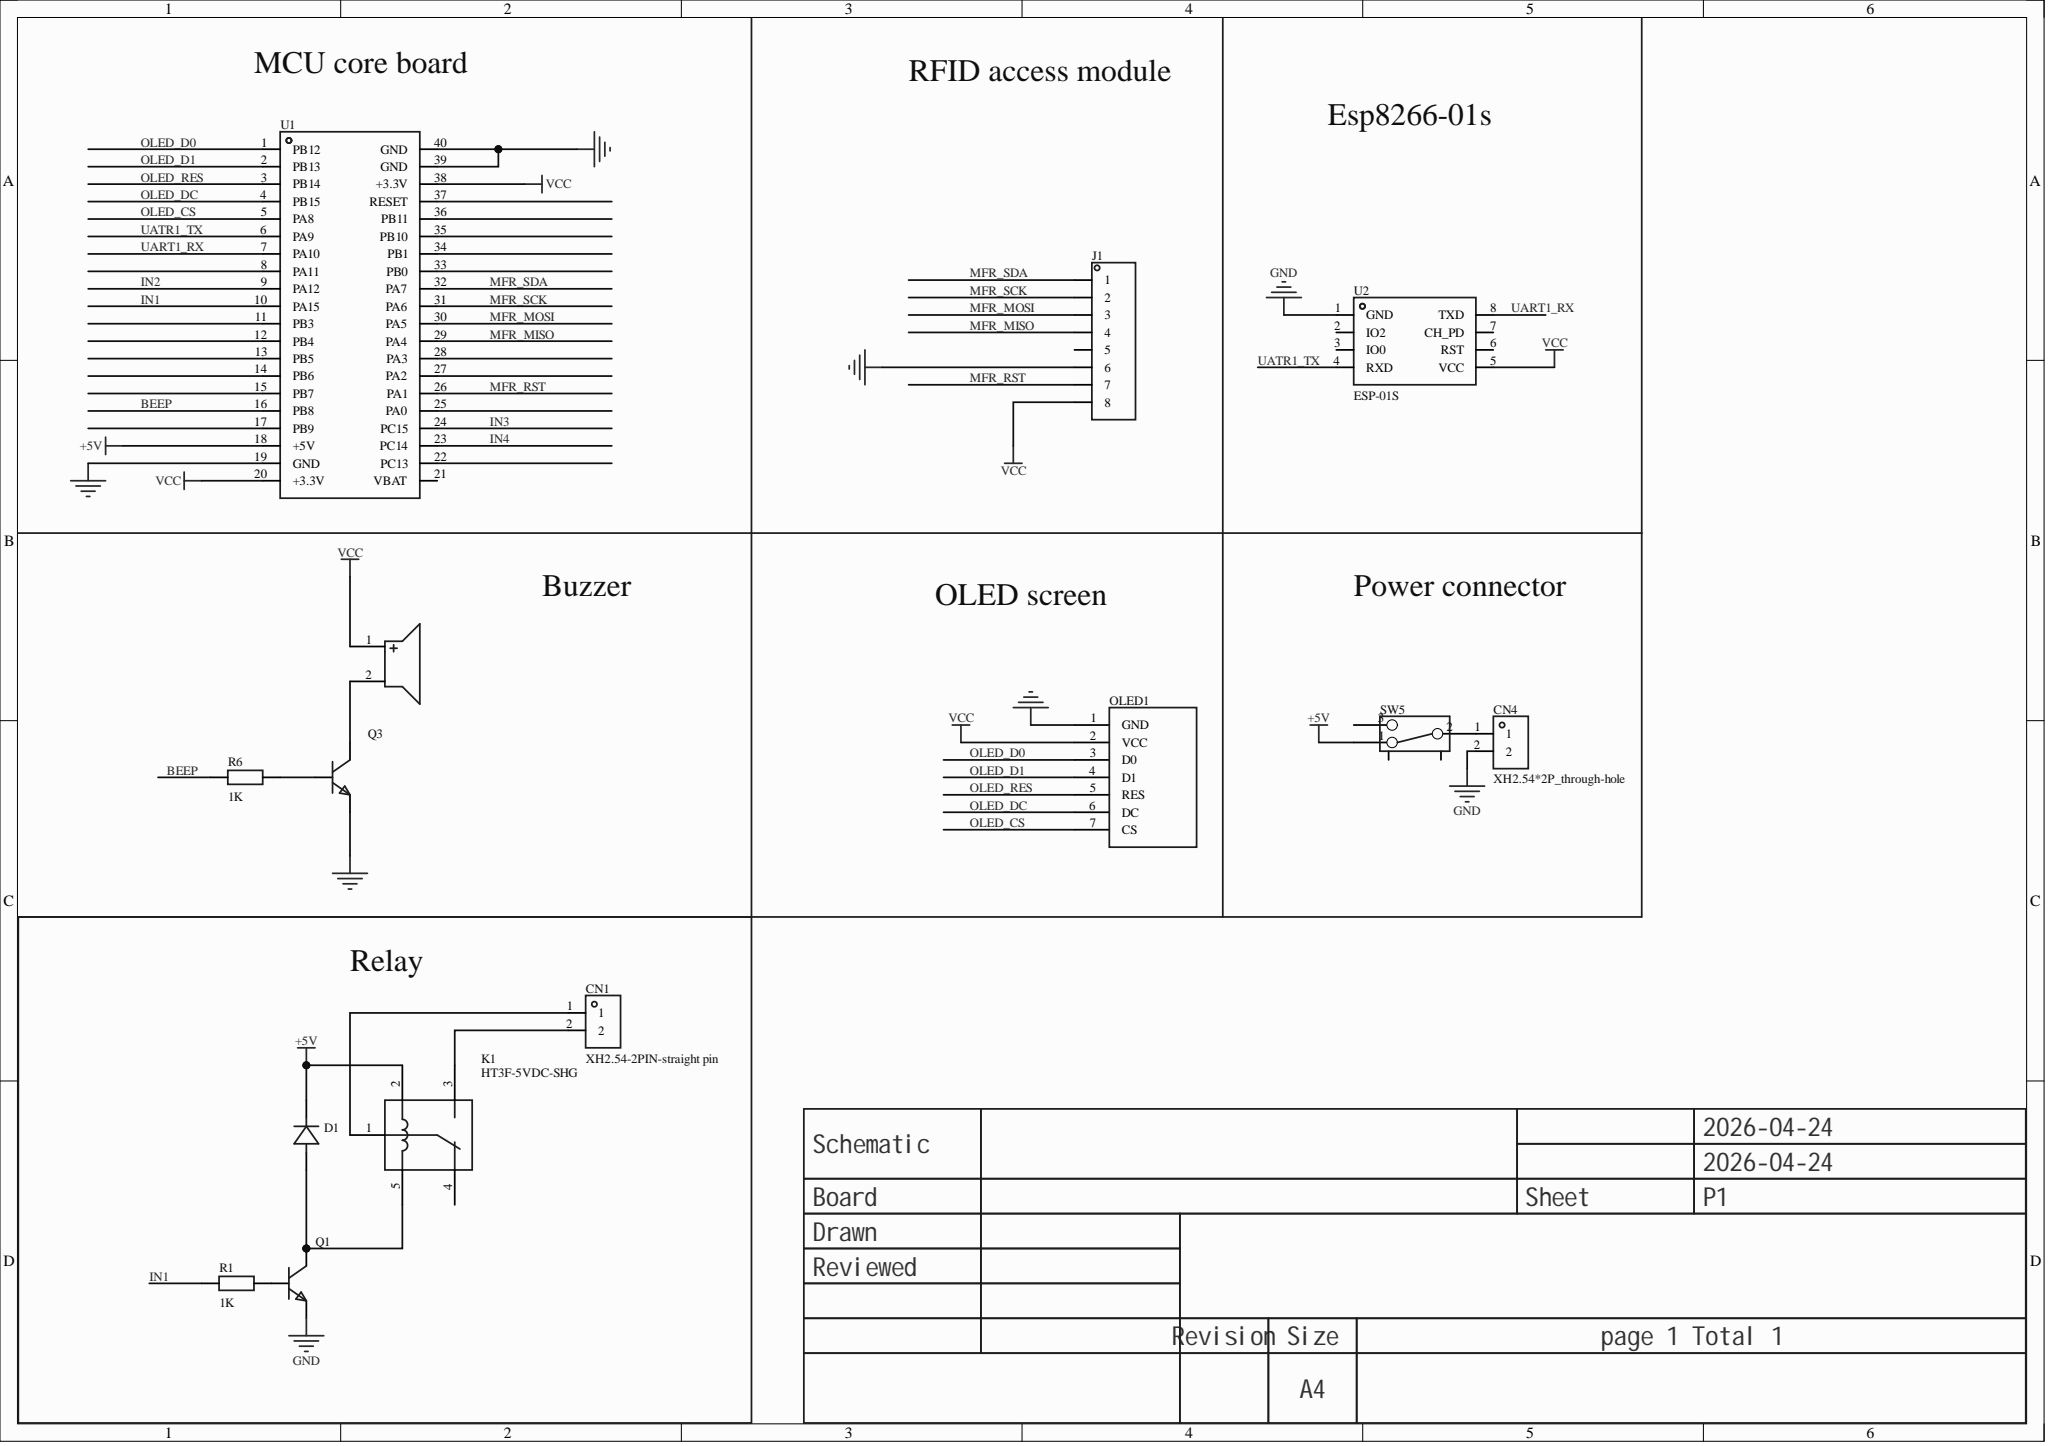Circuit board | Altium Designer | 14 parts | 24 nets
Bill of materials:
Comment,Description,Designator,Footprint,LibRef,Quantity
"2.7kHz","Drive: passive (external drive); type: electromagnetic; frequency: 2.7kHz; SPL: 85dB;","BUZZER1","BUZ-TH_BD9.0-P4.00-D0.6-FD","QMB-09B-03","1"
"XH2.54-2PIN-straight pin","","CN1","CONN-TH_XH2.54-2P","XH2.54-2PIN-直针","1"
"XH2.54*2P_through-hole","","CN4","CONN-TH_2P-P2.50-XH2.54-2P","XH2.54*2P_直插","1"
"","","D1","DO_1N4007","D_1N4007A","1"
"","","J1","HDR-TH_8P-P2.54-V-M","HDR-M_2.54_1x8P","1"
"HT3F-5VDC-SHG","Coil voltage: 5V; contact form: changeover: 1C (SPDT); contact rating (resistive load): 10A@120VAC; 10A@277VAC; 10A@30VDC; max switching voltage: -; max switching current: -","K1","RELAY-TH_HT3F-DCXX-X-X","HT3F-5VDC-SHG","1"
"","","OLED1","0.96OLED","0.96OLED","1"
"","","Q1","S8050_SOT-23","S8050_SOT_NPN","1"
"","","Q3","S8050_TO_92","S8050_TO_NPN","1"
"1K","","R1","R0603","Res_0603","1"
"1K","","R6","Res_1/8W","Res_AXIAL-1/8W","1"
"","","SW5","拨动开关","拨动开关_正","1"
"LCKFB-DKX-STM32F103C8T6","","U1","CONN-TH_L53.3-W22.9_STM32F103C8T6-CARD","LCKFB-DKX-STM32F103C8T6","1"
"ESP-01S","","U2","WIFIM-TH_ESP-01S","ESP-01S_C111009","1"
Netlist (Protel format):
[
BUZZER1
BUZ-TH_BD9.0-P4.00-D0.6-FD
2.7kHz



]
[
CN1
CONN-TH_XH2.54-2P
XH2.54-2PIN-straight pin



]
[
CN4
CONN-TH_2P-P2.50-XH2.54-2P
XH2.54*2P_through-hole



]
[
D1
DO_1N4007




]
[
J1
HDR-TH_8P-P2.54-V-M




]
[
K1
RELAY-TH_HT3F-DCXX-X-X
HT3F-5VDC-SHG



]
[
OLED1
0.96OLED




]
[
Q1
S8050_SOT-23




]
[
Q3
S8050_TO_92




]
[
R1
R0603
1K



]
[
R6
Res_1/8W
1K



]
[
SW5
拨动开关




]
[
U1
CONN-TH_L53.3-W22.9_STM32F103C8T6-CARD
LCKFB-DKX-STM32F103C8T6



]
[
U2
WIFIM-TH_ESP-01S
ESP-01S



]
(
VCC
BUZZER1-1
J1-8
OLED1-2
U1-20
U1-38
U2-5
)
(
UATR1_TX
U1-6
U2-4
)
(
UART1_RX
U1-7
U2-8
)
(
OLED_RES
OLED1-5
U1-3
)
(
OLED_DC
OLED1-6
U1-4
)
(
OLED_D1
OLED1-4
U1-2
)
(
OLED_D0
OLED1-3
U1-1
)
(
OLED_CS
OLED1-7
U1-5
)
(
NetQ3_2
Q3-2
R6-2
)
(
NetQ1_1
Q1-1
R1-2
)
(
NetD1_2
D1-2
K1-5
Q1-3
)
(
NetCN4_1
CN4-1
SW5-2
)
(
NetCN1_2
CN1-2
K1-3
)
(
NetCN1_1
CN1-1
K1-1
)
(
NetBUZZER1_2
BUZZER1-2
Q3-3
)
(
MFR_SDA
J1-1
U1-32
)
(
MFR_SCK
J1-2
U1-31
)
(
MFR_RST
J1-7
U1-26
)
(
MFR_MOSI
J1-3
U1-30
)
(
MFR_MISO
J1-4
U1-29
)
(
IN1
R1-1
U1-10
)
(
GND
CN4-2
J1-6
OLED1-1
Q1-2
Q3-1
U1-19
U1-39
U1-40
U2-1
)
(
BEEP
R6-1
U1-16
)
(
+5V
D1-1
K1-2
SW5-1
U1-18
)